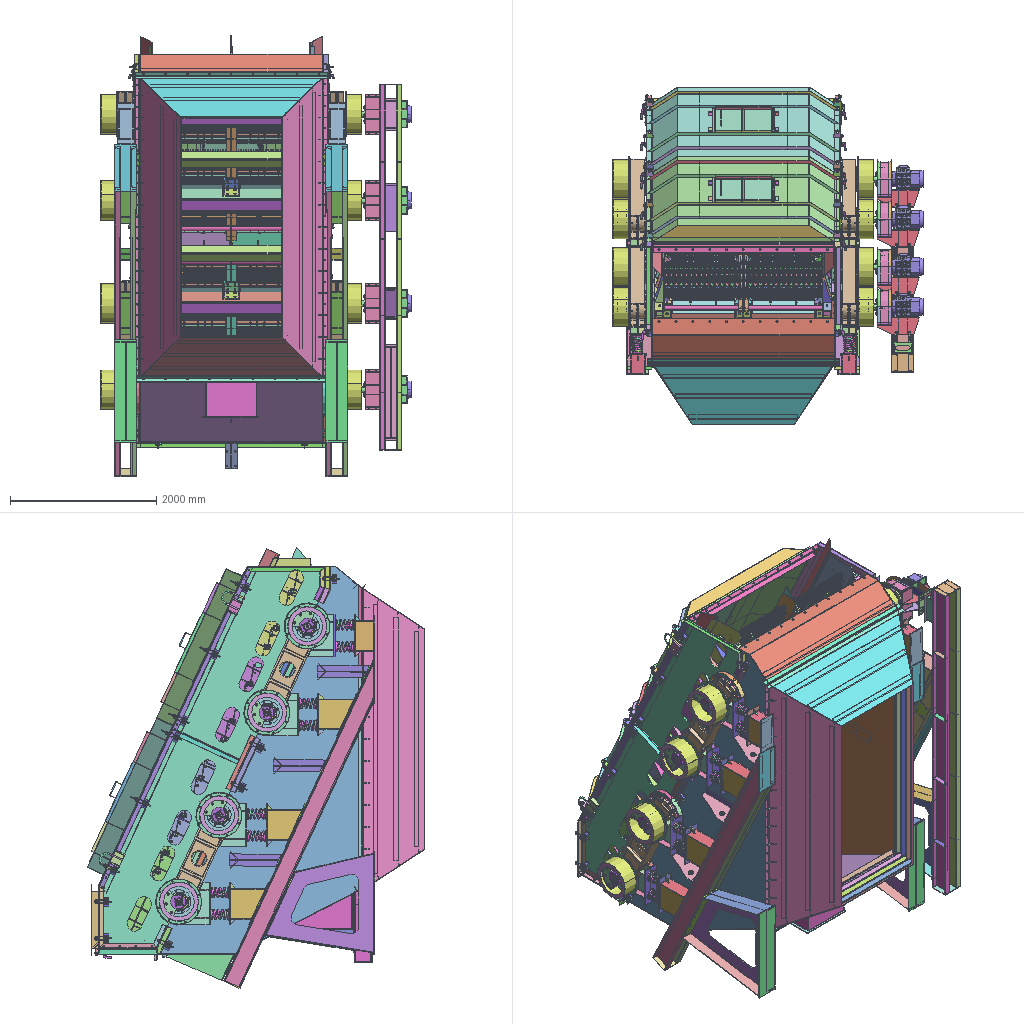Assembly | STEP file | 152 different items | 6490 placed | box 4240 x 4616 x 6023 mm
Parts list (item | name | quantity | parent item | size | volume):
1 | Side plate assembly 2_Default<As machined> | x2 | in Lower hopper | 630.687 x 850.025 x 4105 mm | 42475037 mm3
2 | Rear baffle assembly 2_Default<As machined> | x1 | in Lower hopper | 2450 x 950 x 83 mm | 21025838 mm3
3 | Front baffle assembly 2_Default<As machined> | x1 | in Lower hopper | 2450 x 950 x 83 mm | 21006283 mm3
4 | Angle steel L63X63X8-2626_Default<As machined> | x2 | in Lower hopper | 2626 x 63 x 63 mm | 2498543 mm3
5 | Screen frame side plate assembly_Default<As machined> | x1 | in Upper hopper assembly | 5295 x 2809 x 83 mm | 63364081 mm3
6 | Mirror screen frame side plate assembly_Default<As machined><As machined> | x1 | in Upper hopper assembly | 5295 x 2809 x 83 mm | 63364081 mm3
7 | Positioning angle steel_Default<As machined> | x1 | in Upper hopper assembly | 83 x 58 x 2484 mm | 2642976 mm3
8 | Edge support_Default<As machined> | x3 | in Upper hopper assembly | 168.631 x 720.909 x 332 mm | 2997743 mm3
9 | Mirror edge support_Default<As machined><As machined> | x3 | in Upper hopper assembly | 168.631 x 720.909 x 332 mm | 2997743 mm3
10 | Front baffle_Default<As machined> | x1 | in Upper hopper assembly | 304.499 x 630.195 x 2626 mm | 17251422 mm3
11 | Upper hopper rear baffle_Default<As machined> | x1 | in Upper hopper assembly | 1001 x 2838 x 2626 mm | 60427980 mm3
12 | Screen frame rear support_Default<As machined> | x1 | in Upper hopper assembly | 426.209 x 826.5 x 160 mm | 3581140 mm3
13 | Angle steel L160X60X10-2484_Default<As machined> | x3 | in Upper hopper assembly | 2484 x 226.274 x 118.827 mm | 7825020 mm3
14 | Maintenance pipe_Default<As machined> | x1 | in Hopper assembly | 740 x 860 x 475 mm | 8939485 mm3
15 | Door_Default<As machined> | x1 | in Hopper assembly | 740 x 860 x 74 mm | 3877047 mm3
16 | GN 128.2-120-A41201611203204 | x2 | in Hopper assembly | 20 x 120 x 16 mm | 25167 mm3
17 | Rubber pad_Default<As machined> | x32 | in Spring seat assembly, Spring seat assembly 2 | 160 x 160 x 8 mm | 104144 mm3
18 | Spring lower seat 1_Default<As machined> | x6 | in Spring seat assembly | 580.577 x 601.953 x 230 mm | 9576180 mm3
19 | Helical spring_22X120X280 stiffness 222 | x16 | in Spring seat assembly, Spring seat assembly 2 | 142 x 142 x 244.587 mm | 741236 mm3
20 | Spring upper seat (I)_Default<As machined> | x8 | in Spring seat assembly, Spring seat assembly 2 | 580.577 x 439.316 x 230 mm | 6180967 mm3
21 | Spring lower seat 2_Default<As machined> | x2 | in Spring seat assembly 2 | 575.505 x 341 x 230 mm | 7946213 mm3
22 | _1-QC-408710.step | x27 | in Horizontal tension series latch quick clamp [QC-408710].step | 62 x 37 x 74.9 mm | 22748 mm3
23 | _2-QC-408710.step | x27 | in Horizontal tension series latch quick clamp [QC-408710].step | 60 x 71.267 x 120.088 mm | 53013 mm3
24 | _3-QC-408710.step | x27 | in Horizontal tension series latch quick clamp [QC-408710].step | 57.17 x 14.63 x 155.83 mm | 19518 mm3
25 | _4-QC-408710.step | x27 | in Horizontal tension series latch quick clamp [QC-408710].step | 28 x 37.92 x 40 mm | 9998 mm3
26 | Part 5 | x30 | in Horizontal tension series latch quick clamp [QC-408710], Rear baffle assembly | 126 x 61 x 55 mm | 39850 mm3
27 | Lower channel steel_Default<As machined> | x2 | in Screen frame component assembly | 4891 x 283.464 x 300 mm | 35069262 mm3
28 | Leg_Default<As machined> | x2 | in Screen frame component assembly | 1400 x 1507 x 300 mm | 26750230 mm3
29 | Side plate_Default<As machined> | x1 | in Side plate assembly | 6040 x 1090 x 73 mm | 39402271 mm3
30 | Part 4_Default<As machined> | x1 | in Side plate assembly | 6040 x 1090 x 81 mm | 13497618 mm3
31 | Part 5_Default<As machined> | x14 | in Side plate assembly, Feed inlet assembly, Rear baffle assembly | 82 x 30 x 10 mm | 22938 mm3
32 | Hanger_Default<As machined> | x2 | in Side plate assembly | 190 x 295 x 20 mm | 209555 mm3
33 | Mirror side plate_Default<As machined><As machined> | x1 | in Mirror side plate assembly | 6040 x 1090 x 73 mm | 39402271 mm3
34 | Mirror part 4_Default<As machined> | x1 | in Mirror side plate assembly | 6040 x 1090 x 81 mm | 13497621 mm3
35 | Mirror part 5_Default<As machined><As machined> | x4 | in Mirror side plate assembly | 82 x 30 x 10 mm | 22938 mm3
36 | Mirror hanger_Default<As machined><As machined> | x2 | in Mirror side plate assembly | 190 x 295 x 20 mm | 209555 mm3
37 | Connecting beam 1_Default<As machined> | x1 | in Screen box assembly | 214 x 150.815 x 2484 mm | 9468856 mm3
38 | Connecting beam 2_Default<As machined> | x1 | in Screen box assembly | 2484 x 75 x 180 mm | 5664884 mm3
39 | Connecting beam 3_Default<As machined> | x1 | in Screen box assembly | 255.713 x 102 x 2484 mm | 8118407 mm3
40 | Feed inlet flange_Default<As machined> | x1 | in Feed inlet assembly | 1960 x 960 x 10 mm | 4768318 mm3
41 | Bottom plate 6_Default<As machined> | x1 | in Feed inlet assembly | 934 x 2650 x 6 mm | 6458664 mm3
42 | Liner plate_Default<As machined> | x1 | in Feed inlet assembly | 260 x 1764 x 16 mm | 7243869 mm3
43 | Rear bottom plate_Default<As machined> | x1 | in Feed inlet assembly | 260 x 1784 x 10 mm | 4607815 mm3
44 | Plate 1784X80X8_Default<As machined> | x2 | in Feed inlet assembly | 1784 x 100 x 8 mm | 1427200 mm3
45 | Part 8 | x2 | in Feed inlet assembly | 208 x 768 x 8 mm | 1182208 mm3
46 | GB/T 70.3-2000 hex socket countersunk screw M16×50 (8.8 grade) | x12 | in Feed inlet assembly | 50 x 33.6 x 33.6 mm | 12258 mm3
47 | GB/T 95-2002 flat washer, grade C 16×3 (steel) | x52 | in Feed inlet assembly, Screen box assembly, Exciter assembly | 30 x 3 x 30 mm | 1399 mm3
48 | GB/T 93-1987 standard spring washer (assembly) 16×4.1 (65Mn) | x52 | in Feed inlet assembly, Screen box assembly, Exciter assembly | 24.356 x 24.313 x 4.1 mm | 1031 mm3
49 | GB/T 41-20001 hex nut, grade C, M16 (4 grade) | x20 | in Feed inlet assembly, Screen box assembly | 26.17 x 22.664 x 15.9 mm | 3864 mm3
50 | Rear baffle_Default<As machined> | x1 | in Rear baffle assembly | 150 x 800 x 2650 mm | 24404542 mm3
51 | Seal cover 2_Default<As machined> | x1 | in Screen box assembly | 2723 x 292.121 x 2296 mm | 30393848 mm3
52 | Seal cover 1_Default<As machined> | x1 | in Screen box assembly | 2723 x 286.121 x 2250 mm | 29731618 mm3
53 | Manhole door_Default<As machined> | x2 | in Screen box assembly | 840 x 840 x 140 mm | 3861650 mm3
54 | _PDHFA1-75.step | x4 | in Welded hinge, square, A series [PDHFA-75].step | 29.25 x 8.5 x 75 mm | 5922 mm3
55 | _PDHFA2-75.step | x4 | in Welded hinge, square, A series [PDHFA-75].step | 29.25 x 8.5 x 75 mm | 5070 mm3
56 | GB/T 5781-2000 hex head bolt, fully threaded, grade C M16×45 (3.6 grade) | x8 | in Screen box assembly | 55 x 27.713 x 24 mm | 13928 mm3
57 | Screen plate bracket (middle 1)_Default<As machined> | x1 | in Screen plate bracket in | 3120 x 451.736 x 230 mm | 29285833 mm3
58 | Screen plate bracket (edge)_Default<As machined> | x4 | in Screen plate bracket in, Screen plate bracket out | 2750 x 152 x 230 mm | 16995025 mm3
59 | Square tube 120X120X8-1079_Default<As machined> | x8 | in Screen plate bracket in, Screen plate bracket out | 1079 x 120 x 120 mm | 3686687 mm3
60 | Gusset plate 1_Default<As machined> | x32 | in Screen plate bracket in, Screen plate bracket out | 60 x 100 x 12 mm | 54600 mm3
61 | - | x4 | in Screen plate bracket in, Screen plate bracket out | 2404 x 70 x 70 mm | 3745985 mm3
62 | Beam guard plate_Default<As machined> | x8 | in Screen plate bracket in, Screen plate bracket out | 305.019 x 262.777 x 850 mm | 2327560 mm3
63 | GB/T 5783-2000 hex head bolt, fully threaded M10×45 (5.6 grade) | x64 | in Screen plate bracket in, Screen plate bracket out, Exciter assembly | 31.4 x 18.475 x 16 mm | 3346 mm3
64 | GB/T 93-1987 standard spring washer (assembly) 10×2.6 (65Mn) | x64 | in Screen plate bracket in, Screen plate bracket out, Exciter assembly | 15.372 x 15.344 x 2.6 mm | 261.313 mm3
65 | GB/T 95-2002 flat washer, grade C 10×2 (steel) | x64 | in Screen plate bracket in, Screen plate bracket out, Exciter assembly | 20 x 2 x 20 mm | 438.252 mm3
66 | Screen plate bracket (middle 2)_Default<As machined> | x1 | in Screen plate bracket out | 2936 x 451.736 x 230 mm | 28253471 mm3
67 | Motor bracket lower channel steel_Default<As machined> | x1 | in Motor bracket assembly | 5000 x 250 x 300 mm | 37542692 mm3
68 | Motor bracket leg_Default<As machined> | x1 | in Motor bracket assembly | 1300 x 1259 x 300 mm | 22043993 mm3
69 | Motor base_Default<As machined> | x4 | in Assembly 3, Motor bracket assembly | 572.5 x 250 x 550 mm | 5315088 mm3
70 | Motor lower seat 1_Default<As machined> | x3 | in Assembly 3 | 436 x 591.846 x 300 mm | 6753859 mm3
71 | GB/T901-1988 double-end stud, grade B, M24×300 | x12 | in Assembly 3 | 300 x 24 x 24 mm | 120071 mm3
72 | GB/T41-20001 hex nut, grade C, M24 | x64 | in Assembly 3, Motor bracket assembly | 39.55 x 34.251 x 22.3 mm | 12527 mm3
73 | Coupling guard_Default<As machined> | x4 | in Assembly 3, Motor bracket assembly | 550 x 522 x 200 mm | 1395194 mm3
74 | Motor base support channel steel_Default<As machined> | x1 | in Motor bracket assembly | 3569 x 291.917 x 300 mm | 27407962 mm3
75 | Motor lower seat 2_Default<As machined> | x1 | in Motor bracket assembly | 436 x 154.533 x 300 mm | 3621040 mm3
76 | GB/T901-1988 double-end stud, grade B, M24×200 | x4 | in Motor bracket assembly | 200 x 24 x 24 mm | 86144 mm3
77 | Rectangular tube | x4 | in Rectangular tube beam | 239 x 320 x 2600 mm | 50963884 mm3
78 | Flange | x8 | in Rectangular tube beam | 34 x 476 x 476 mm | 2924692 mm3
79 | Plate 510x230x16 | x4 | in Rectangular tube beam | 510 x 2414 x 16 mm | 5441904 mm3
80 | GB/T 5783-2000 hex head bolt, fully threaded, M20×40 (5.6 grade) | x8 | in Rectangular tube beam | 52.5 x 34.641 x 30 mm | 22112 mm3
81 | Rib 9 | x16 | in Rectangular tube beam | 60 x 60 x 12 mm | 27600 mm3
82 | Rib 7 | x16 | in Rectangular tube beam | 150 x 60 x 12 mm | 77400 mm3
83 | Reinforcing plate 4 | x24 | in Rectangular tube beam | 230 x 230 x 12 mm | 600871 mm3
84 | Rib 6 | x48 | in Rectangular tube beam | 123 x 230 x 12 mm | 222480 mm3
85 | Drive shaft | x4 | in Exciter assembly | 3402 x 140 x 140 mm | 19524168 mm3
86 | Oil retaining ring | x8 | in Exciter assembly | 41.5 x 216 x 216 mm | 640315 mm3
87 | GB/T1096-1979 plain key, type A, 24×90 | x8 | in Exciter assembly | 90 x 24 x 14 mm | 28453 mm3
88 | End disc | x8 | in Exciter assembly | 620 x 620 x 4 mm | 989174 mm3
89 | Labyrinth cover | x8 | in Exciter assembly | 65 x 227.5 x 227.5 mm | 634652 mm3
90 | Offset block | x8 | in Offset block assembly | 424.352 x 335 x 125 mm | 6174570 mm3
91 | Part 7 | x24 | in Offset block assembly | 389.711 x 169 x 20 mm | 776785 mm3
92 | GB/T 5780-2000 hex head bolt, grade C, M20×120 (3.6 grade) | x24 | in Offset block assembly | 132.5 x 34.641 x 30 mm | 47244 mm3
93 | GB/T 93-1987 standard spring washer (assembly) 20×5 (65Mn) | x32 | in Offset block assembly, Exciter assembly | 30.149 x 30.097 x 5 mm | 1905 mm3
94 | Through-hole cover | x8 | in Exciter assembly | 49 x 330 x 330 mm | 1508672 mm3
95 | Shaft end baffle | x8 | in Exciter assembly | 20 x 95 x 95 mm | 108579 mm3
96 | Taper sleeve | x8 | in Exciter assembly | 120 x 95 x 94.958 mm | 185425 mm3
97 | Bearing housing | x4 | in Exciter assembly | 1820 x 234 x 460 mm | 47518256 mm3
98 | GB/T288-94 spherical roller bearing 22324C_1 | x8 | in Exciter assembly | 86 x 260 x 260 mm | 2801542 mm3
99 | JB1091-1991 skeleton-type vacuum rubber seal ring 140 | x8 | in Exciter assembly | 170 x 16 x 170 mm | 62160 mm3
100 | GB/T 5786-2000 hex head bolt, fine thread, fully threaded, grade A and B, M24×60 (5.6 grade) | x8 | in Exciter assembly | 75 x 41.569 x 36 mm | 43647 mm3
101 | GB/T 93-1987 standard spring washer (assembly) 24×6 (65Mn) | x72 | in Exciter assembly | 36.439 x 36.377 x 6 mm | 3321 mm3
102 | Guard cover | x8 | in Exciter assembly | 620 x 620 x 220 mm | 2105294 mm3
103 | GB/T 5780-2000 hex head bolt, grade C, M24×100 (3.6 grade) | x64 | in Exciter assembly | 115 x 41.569 x 36 mm | 61742 mm3
104 | GB/T 95-2002 flat washer, grade C 24×4 (steel) | x64 | in Exciter assembly | 44 x 4 x 44 mm | 3958 mm3
105 | GB/T 41-20001 hex nut, grade C, M24 (4 grade) | x64 | in Exciter assembly | 39.55 x 34.251 x 22.3 mm | 12527 mm3
106 | GB/T 5781-2000 hex head bolt, fully threaded, grade C, M12×45 (3.6 grade) | x64 | in Exciter assembly | 52.5 x 20.785 x 18 mm | 7141 mm3
107 | GB/T 93-1987 standard spring washer (assembly) 12×3.1 (65Mn) | x64 | in Exciter assembly | 18.367 x 18.334 x 3.1 mm | 444.091 mm3
108 | GB/T 41-20001 hex nut, grade C, M10 (4 grade) | x32 | in Exciter assembly | 17.59 x 15.233 x 9.5 mm | 1159 mm3
109 | Coupling | x4 | in Exciter assembly | 157 x 250 x 250 mm | 2335528 mm3
110 | GB/T 5780-2000 hex head bolt, grade C, M20×80 (3.6 grade) | x8 | in Exciter assembly | 92.5 x 34.641 x 30 mm | 34678 mm3
111 | GB/T 95-2002 flat washer, grade C 20×3 (steel) | x8 | in Exciter assembly | 37 x 3 x 37 mm | 2085 mm3
112 | Coupling 2 | x4 | in Exciter assembly | 104 x 250 x 250 mm | 1439037 mm3
113 | Coupling rubber strip | x16 | in Exciter assembly | 129 x 167.5 x 80 mm | 367054 mm3
114 | Pressing pad | x32 | in Exciter assembly | 60 x 60 x 10 mm | 25730 mm3
115 | GB/T 5780-2000 hex head bolt, grade C, M16×65 (3.6 grade) | x32 | in Exciter assembly | 75 x 27.713 x 24 mm | 17949 mm3
116 | IM B3 H63-132 variable-frequency motor [YVF2-132S2-4-B3]_YVF2-132S2-4-B3 | x4 | in 1233 | 270 x 315 x 510 mm | 20221478 mm3
117 | Grid blind plate_Default<As machined> | x2 | in Bar screen plate 1 | 874.382 x 165 x 1059 mm | 15878057 mm3
118 | Positioning slot assembly 1_Default<As machined> | x30 | in Bar screen assembly 1 | 100 x 92 x 1069 mm | 2012408 mm3
119 | - | x930 | in Bar screen assembly 1 | 10 x 10 x 340 mm | 26704 mm3
120 | - | x930 | in Bar screen assembly 1 | 10 x 10 x 310 mm | 24347 mm3
121 | - | x2610 | in Bar screen assembly 1 | 8 x 8 x 310 mm | 15582 mm3
122 | Pressure plate 1069X36X6_Default<As machined> | x30 | in Bar screen assembly 1 | 1069 x 6 x 36 mm | 230904 mm3
123 | GB/T5783-2000 hex head bolt, fully threaded M10×45 | x180 | in Bar screen assembly 1 | 51.4 x 18.475 x 16 mm | 4917 mm3
124 | Rear baffle 1079X402X8_Default<As machined> | x2 | in Bar screen plate 1 | 1079 x 402 x 8 mm | 3470064 mm3
125 | - | x84 | in Bar screen plate 1, Bar screen plate 2, Bar screen plate 3, Bar screen plate 4 | 36 x 36 x 280 mm | 87085 mm3
126 | - | x28 | in Bar screen plate 1, Bar screen plate 2, Bar screen plate 3, Bar screen plate 4 | 16 x 16 x 1069 mm | 214935 mm3
127 | Connecting plate assembly 1_Default<As machined> | x4 | in Bar screen plate 1 | 725.342 x 86.845 x 24 mm | 319823 mm3
128 | Edge plate 1_Default<As machined> | x1 | in Bar screen plate 1 | 1555 x 210 x 35 mm | 3116927 mm3
129 | Edge plate 2_Default<As machined> | x1 | in Bar screen plate 1 | 130 x 532.359 x 1587 mm | 10246266 mm3
130 | Rubber plate 1_Default<As machined> | x2 | in Bar screen plate 1 | 1355 x 250 x 8 mm | 2297597 mm3
131 | Mirror edge plate 1_Default<As machined><As machined> | x1 | in Bar screen plate 1 | 1555 x 210 x 35 mm | 3116927 mm3
132 | Mirror edge plate 2_Default<As machined><As machined> | x1 | in Bar screen plate 1 | 130 x 532.359 x 1587 mm | 10246266 mm3
133 | Connecting plate assembly 2_Default<As machined> | x4 | in Bar screen plate 2 | 1223 x 86.845 x 24 mm | 635186 mm3
134 | Edge plate 3_Default<As machined> | x1 | in Bar screen plate 2 | 1554 x 210 x 35 mm | 2937527 mm3
135 | Edge plate 4_Default<As machined> | x1 | in Bar screen plate 2 | 207.636 x 532.359 x 1552 mm | 10466658 mm3
136 | Rubber plate 2_Default<As machined> | x6 | in Bar screen plate 2, Bar screen plate 3, Bar screen plate 4 | 1374 x 250 x 8 mm | 2740611 mm3
137 | Pressure plate 2_Default<As machined> | x6 | in Bar screen plate 2, Bar screen plate 3, Bar screen plate 4 | 1374 x 40 x 4 mm | 216145 mm3
138 | Bent plate 1_Default<As machined> | x1 | in Bar screen plate 2 | 330 x 204.897 x 1059 mm | 4219235 mm3
139 | Liner plate 1_Default<As machined> | x2 | in Bar screen plate 2 | 330 x 1049 x 8 mm | 2695509 mm3
140 | Mirror edge plate 3_Default<As machined><As machined> | x1 | in Bar screen plate 2 | 1554 x 210 x 35 mm | 2937527 mm3
141 | Mirror bent plate 1_Default<As machined><As machined> | x1 | in Bar screen plate 2 | 330 x 204.897 x 1059 mm | 4219235 mm3
142 | Mirror edge plate 4_Default<As machined><As machined> | x1 | in Bar screen plate 2 | 207.636 x 532.359 x 1552 mm | 10466658 mm3
143 | Edge plate 5_Default<As machined> | x1 | in Bar screen plate 3 | 1374 x 260 x 35 mm | 3099117 mm3
144 | Edge plate 6_Default<As machined> | x1 | in Bar screen plate 3 | 130 x 532.359 x 1374 mm | 9676363 mm3
145 | Connecting plate assembly 3_Default<As machined> | x4 | in Bar screen plate 3 | 1250 x 86.845 x 24 mm | 582349 mm3
146 | Mirror edge plate 5_Default<As machined><As machined> | x1 | in Bar screen plate 3 | 1374 x 260 x 35 mm | 3099117 mm3
147 | Mirror edge plate 6_Default<As machined><As machined> | x1 | in Bar screen plate 3 | 130 x 532.359 x 1374 mm | 9676363 mm3
148 | Edge plate 7_Default<As machined> | x1 | in Bar screen plate 4 | 1511 x 260 x 35 mm | 3690417 mm3
149 | Edge plate 8_Default<As machined> | x1 | in Bar screen plate 4 | 130 x 532.359 x 1511 mm | 9898489 mm3
150 | Bar screen plate 4_Default<As machined> | x4 | in Bar screen plate 4 | 1234 x 86.845 x 24 mm | 638578 mm3
151 | Mirror edge plate 7_Default<As machined><As machined> | x1 | in Bar screen plate 4 | 1511 x 260 x 35 mm | 3690417 mm3
152 | Mirror edge plate 8_Default<As machined><As machined> | x1 | in Bar screen plate 4 | 130 x 532.359 x 1511 mm | 9898489 mm3
Placements (level | parent | child | x y z in mm | rotation matrix by rows), first 266 of 6622 lines:
1 | 1233 | Screen frame component assembly | -0.0 -0.0 -0.0 | 1 0 0 0 1 0 0 0 1
2 | Screen frame component assembly | Hopper assembly | -0.0 -0.0 -0.0 | 1 0 0 0 1 0 0 0 1
3 | Hopper assembly | Lower hopper | -0.0 -0.0 -0.0 | 1 0 0 0 1 0 0 0 1
4 | Lower hopper | Side plate assembly 2_Default<As machined> | 1313.0 -8.0 0.0 | 1 0 0 0 1 0 0 0 1
4 | Lower hopper | Rear baffle assembly 2_Default<As machined> | 0.0 -850.025 1509.541 | -1 0 0 0 0.8385 0.545 0 0.545 -0.8385
4 | Lower hopper | Front baffle assembly 2_Default<As machined> | 0.0 -850.025 -1509.541 | 1 0 0 0 0.8385 0.545 0 -0.545 0.8385
4 | Lower hopper | Side plate assembly 2_Default<As machined> | -1313.0 -8.0 0.0 | -1 0 0 0 1 0 0 0 -1
4 | Lower hopper | Angle steel L63X63X8-2626_Default<As machined> | 0.0 -0.0 2062.041 | 1 0 0 0 -0.545 -0.8385 0 0.8385 -0.545
4 | Lower hopper | Angle steel L63X63X8-2626_Default<As machined> | -0.0 -0.0 -2062.041 | -1 0 0 0 -0.545 -0.8385 0 -0.8385 0.545
3 | Hopper assembly | Upper hopper assembly | -4045.416 1401.429 -250.506 | 0 0 1 0 1 0 -1 0 0
4 | Upper hopper assembly | Screen frame side plate assembly_Default<As machined> | 1791.123 -1401.429 5295.416 | 1 0 0 0 1 0 0 0 1
4 | Upper hopper assembly | Mirror screen frame side plate assembly_Default<As machined><As machined> | 1791.123 -1401.429 2795.416 | 1 0 0 0 1 0 0 0 1
4 | Upper hopper assembly | Positioning angle steel_Default<As machined> | -0.0 -0.0 -0.0 | 1 0 0 0 1 0 0 0 1
4 | Upper hopper assembly | Edge support_Default<As machined> | -1176.285 -781.042 2791.416 | -1 -0.006557 0 -0.006557 1 0 0 0 -1
4 | Upper hopper assembly | Edge support_Default<As machined> | 110.808 -180.861 2791.416 | -1 -0.006557 0 -0.006557 1 0 0 0 -1
4 | Upper hopper assembly | Edge support_Default<As machined> | 1397.9 419.32 2791.416 | -1 -0.006557 0 -0.006557 1 0 0 0 -1
4 | Upper hopper assembly | Mirror edge support_Default<As machined><As machined> | 1397.9 419.32 5299.416 | -1 -0.006557 0 -0.006557 1 0 0 0 -1
4 | Upper hopper assembly | Mirror edge support_Default<As machined><As machined> | 110.808 -180.861 5299.416 | -1 -0.006557 0 -0.006557 1 0 0 0 -1
4 | Upper hopper assembly | Mirror edge support_Default<As machined><As machined> | -1176.285 -781.042 5299.416 | -1 -0.006557 0 -0.006557 1 0 0 0 -1
4 | Upper hopper assembly | Front baffle_Default<As machined> | -2611.106 -810.792 4045.416 | -1 0 0 0 1 0 0 0 -1
4 | Upper hopper assembly | Upper hopper rear baffle_Default<As machined> | 2684.309 1407.529 4045.416 | 1 0 0 0 1 0 0 0 1
4 | Upper hopper assembly | Screen frame rear support_Default<As machined> | 3042.855 530.716 4045.416 | -0.9011 -0.4335 0 -0.4335 0.9011 0 0 0 -1
4 | Upper hopper assembly | Angle steel L160X60X10-2484_Default<As machined> | -1175.446 -909.02 4045.416 | 0 -1 -0.006557 0 -0.006557 1 -1 0 0
4 | Upper hopper assembly | Angle steel L160X60X10-2484_Default<As machined> | 111.647 -308.839 4045.416 | 0 -1 -0.006557 0 -0.006557 1 -1 0 0
4 | Upper hopper assembly | Angle steel L160X60X10-2484_Default<As machined> | 1398.74 291.343 4045.416 | 0 -1 -0.006557 0 -0.006557 1 -1 0 0
3 | Hopper assembly | Maintenance pipe_Default<As machined> | -0.0 541.628 -2591.349 | 1 0 0 0 1 0 0 0 1
3 | Hopper assembly | Door_Default<As machined> | -0.0 541.628 -2591.349 | -1 0 0 0 1 0 0 0 -1
3 | Hopper assembly | GN 128.2-120-A41201611203204 | 358.0 823.128 -2589.349 | -0.6 0 0.8 0 -1 0 0.8 0 0.6
3 | Hopper assembly | GN 128.2-120-A41201611203204 | 358.0 260.128 -2589.349 | -0.6 0 0.8 0 -1 0 0.8 0 0.6
2 | Screen frame component assembly | Spring seat assembly | -1442.0 617.014 337.6 | 0 0 1 0 1 0 -1 0 0
3 | Spring seat assembly | Rubber pad_Default<As machined> | -150.0 -0.0 0.0 | -0.03619 0.9993 0 0 0 1 0.9993 0.03619 0
3 | Spring seat assembly | Spring lower seat 1_Default<As machined> | 0.0 -0.0 -0.0 | -1 0 0 0 1 0 0 0 -1
3 | Spring seat assembly | Helical spring_22X120X280 stiffness 222 | -150.0 2.473 -0.0 | -0.008683 1 0 0 0 1 1 0.008683 0
3 | Spring seat assembly | Helical spring_22X120X280 stiffness 222 | 150 2.473 -0.0061 | -0.008683 -1 0 0 0 1 -1 0.008683 0
3 | Spring seat assembly | Rubber pad_Default<As machined> | 150.0 8.0 0.0 | 0.03619 -0.9993 0 0 0 -1 0.9993 0.03619 -0
3 | Spring seat assembly | Rubber pad_Default<As machined> | -150.0 252.587 0.0 | -0.03619 0.9993 0 0 0 1 0.9993 0.03619 0
3 | Spring seat assembly | Rubber pad_Default<As machined> | 150.0 260.587 0.0 | 0.03619 -0.9993 0 0 0 -1 0.9993 0.03619 -0
3 | Spring seat assembly | Spring upper seat (I)_Default<As machined> | 0.0 260.587 -0.0 | -1 0 0 0 1 0 0 0 -1
2 | Screen frame component assembly | Spring seat assembly | -1442.0 1320.672 -1171.4 | 0 0 1 0 1 0 -1 0 0
3 | Spring seat assembly | Rubber pad_Default<As machined> | -150.0 -0.0 0.0 | -0.03619 0.9993 0 0 0 1 0.9993 0.03619 0
3 | Spring seat assembly | Spring lower seat 1_Default<As machined> | 0.0 -0.0 -0.0 | -1 0 0 0 1 0 0 0 -1
3 | Spring seat assembly | Helical spring_22X120X280 stiffness 222 | -150.0 2.473 -0.0 | -0.008683 1 0 0 0 1 1 0.008683 0
3 | Spring seat assembly | Helical spring_22X120X280 stiffness 222 | 150 2.473 -0.0061 | -0.008683 -1 0 0 0 1 -1 0.008683 0
3 | Spring seat assembly | Rubber pad_Default<As machined> | 150.0 8.0 0.0 | 0.03619 -0.9993 0 0 0 -1 0.9993 0.03619 -0
3 | Spring seat assembly | Rubber pad_Default<As machined> | -150.0 252.587 0.0 | -0.03619 0.9993 0 0 0 1 0.9993 0.03619 0
3 | Spring seat assembly | Rubber pad_Default<As machined> | 150.0 260.587 0.0 | 0.03619 -0.9993 0 0 0 -1 0.9993 0.03619 -0
3 | Spring seat assembly | Spring upper seat (I)_Default<As machined> | 0.0 260.587 -0.0 | -1 0 0 0 1 0 0 0 -1
2 | Screen frame component assembly | Spring seat assembly | -1442.0 1821.487 -2245.4 | 0 0 1 0 1 0 -1 0 0
3 | Spring seat assembly | Rubber pad_Default<As machined> | -150.0 -0.0 0.0 | -0.03619 0.9993 0 0 0 1 0.9993 0.03619 0
3 | Spring seat assembly | Spring lower seat 1_Default<As machined> | 0.0 -0.0 -0.0 | -1 0 0 0 1 0 0 0 -1
3 | Spring seat assembly | Helical spring_22X120X280 stiffness 222 | -150.0 2.473 -0.0 | -0.008683 1 0 0 0 1 1 0.008683 0
3 | Spring seat assembly | Helical spring_22X120X280 stiffness 222 | 150 2.473 -0.0061 | -0.008683 -1 0 0 0 1 -1 0.008683 0
3 | Spring seat assembly | Rubber pad_Default<As machined> | 150.0 8.0 0.0 | 0.03619 -0.9993 0 0 0 -1 0.9993 0.03619 -0
3 | Spring seat assembly | Rubber pad_Default<As machined> | -150.0 252.587 0.0 | -0.03619 0.9993 0 0 0 1 0.9993 0.03619 0
3 | Spring seat assembly | Rubber pad_Default<As machined> | 150.0 260.587 0.0 | 0.03619 -0.9993 0 0 0 -1 0.9993 0.03619 -0
3 | Spring seat assembly | Spring upper seat (I)_Default<As machined> | 0.0 260.587 -0.0 | -1 0 0 0 1 0 0 0 -1
2 | Screen frame component assembly | Spring seat assembly | 1442.0 1821.487 -2245.4 | 0 0 1 0 1 0 -1 0 -0
3 | Spring seat assembly | Rubber pad_Default<As machined> | -150.0 -0.0 0.0 | -0.03619 0.9993 0 0 0 1 0.9993 0.03619 0
3 | Spring seat assembly | Spring lower seat 1_Default<As machined> | 0.0 -0.0 -0.0 | -1 0 0 0 1 0 0 0 -1
3 | Spring seat assembly | Helical spring_22X120X280 stiffness 222 | -150.0 2.473 -0.0 | -0.008683 1 0 0 0 1 1 0.008683 0
3 | Spring seat assembly | Helical spring_22X120X280 stiffness 222 | 150 2.473 -0.0061 | -0.008683 -1 0 0 0 1 -1 0.008683 0
3 | Spring seat assembly | Rubber pad_Default<As machined> | 150.0 8.0 0.0 | 0.03619 -0.9993 0 0 0 -1 0.9993 0.03619 -0
3 | Spring seat assembly | Rubber pad_Default<As machined> | -150.0 252.587 0.0 | -0.03619 0.9993 0 0 0 1 0.9993 0.03619 0
3 | Spring seat assembly | Rubber pad_Default<As machined> | 150.0 260.587 0.0 | 0.03619 -0.9993 0 0 0 -1 0.9993 0.03619 -0
3 | Spring seat assembly | Spring upper seat (I)_Default<As machined> | 0.0 260.587 -0.0 | -1 0 0 0 1 0 0 0 -1
2 | Screen frame component assembly | Spring seat assembly | 1442.0 1320.672 -1171.4 | 0 0 1 0 1 0 -1 0 -0
3 | Spring seat assembly | Rubber pad_Default<As machined> | -150.0 -0.0 0.0 | -0.03619 0.9993 0 0 0 1 0.9993 0.03619 0
3 | Spring seat assembly | Spring lower seat 1_Default<As machined> | 0.0 -0.0 -0.0 | -1 0 0 0 1 0 0 0 -1
3 | Spring seat assembly | Helical spring_22X120X280 stiffness 222 | -150.0 2.473 -0.0 | -0.008683 1 0 0 0 1 1 0.008683 0
3 | Spring seat assembly | Helical spring_22X120X280 stiffness 222 | 150 2.473 -0.0061 | -0.008683 -1 0 0 0 1 -1 0.008683 0
3 | Spring seat assembly | Rubber pad_Default<As machined> | 150.0 8.0 0.0 | 0.03619 -0.9993 0 0 0 -1 0.9993 0.03619 -0
3 | Spring seat assembly | Rubber pad_Default<As machined> | -150.0 252.587 0.0 | -0.03619 0.9993 0 0 0 1 0.9993 0.03619 0
3 | Spring seat assembly | Rubber pad_Default<As machined> | 150.0 260.587 0.0 | 0.03619 -0.9993 0 0 0 -1 0.9993 0.03619 -0
3 | Spring seat assembly | Spring upper seat (I)_Default<As machined> | 0.0 260.587 -0.0 | -1 0 0 0 1 0 0 0 -1
2 | Screen frame component assembly | Spring seat assembly | 1442.0 617.014 337.6 | 0 0 1 0 1 0 -1 0 -0
3 | Spring seat assembly | Rubber pad_Default<As machined> | -150.0 -0.0 0.0 | -0.03619 0.9993 0 0 0 1 0.9993 0.03619 0
3 | Spring seat assembly | Spring lower seat 1_Default<As machined> | 0.0 -0.0 -0.0 | -1 0 0 0 1 0 0 0 -1
3 | Spring seat assembly | Helical spring_22X120X280 stiffness 222 | -150.0 2.473 -0.0 | -0.008683 1 0 0 0 1 1 0.008683 0
3 | Spring seat assembly | Helical spring_22X120X280 stiffness 222 | 150 2.473 -0.0061 | -0.008683 -1 0 0 0 1 -1 0.008683 0
3 | Spring seat assembly | Rubber pad_Default<As machined> | 150.0 8.0 0.0 | 0.03619 -0.9993 0 0 0 -1 0.9993 0.03619 -0
3 | Spring seat assembly | Rubber pad_Default<As machined> | -150.0 252.587 0.0 | -0.03619 0.9993 0 0 0 1 0.9993 0.03619 0
3 | Spring seat assembly | Rubber pad_Default<As machined> | 150.0 260.587 0.0 | 0.03619 -0.9993 0 0 0 -1 0.9993 0.03619 -0
3 | Spring seat assembly | Spring upper seat (I)_Default<As machined> | 0.0 260.587 -0.0 | -1 0 0 0 1 0 0 0 -1
2 | Screen frame component assembly | Spring seat assembly 2 | -1442.0 116.975 1411.6 | 0 0 1 0 1 0 -1 0 0
3 | Spring seat assembly 2 | Rubber pad_Default<As machined> | -150.0 0.0 0.0 | -0.03619 0.9993 0 0 0 1 0.9993 0.03619 0
3 | Spring seat assembly 2 | Spring lower seat 2_Default<As machined> | 0.0 -0.0 -0.0 | -1 0 0 0 1 0 0 0 -1
3 | Spring seat assembly 2 | Helical spring_22X120X280 stiffness 222 | -150.0 2.473 0.0 | -0.008683 1 0 0 0 1 1 0.008683 0
3 | Spring seat assembly 2 | Helical spring_22X120X280 stiffness 222 | 150 2.473 -0.0061 | -0.008683 -1 0 0 0 1 -1 0.008683 0
3 | Spring seat assembly 2 | Rubber pad_Default<As machined> | 150.0 8.0 0.0 | 0.03619 -0.9993 0 0 0 -1 0.9993 0.03619 -0
3 | Spring seat assembly 2 | Rubber pad_Default<As machined> | 150.0 260.587 -0.0 | 0.03619 -0.9993 0 0 0 -1 0.9993 0.03619 -0
3 | Spring seat assembly 2 | Rubber pad_Default<As machined> | -150.0 252.587 0.0 | -0.03619 0.9993 0 0 0 1 0.9993 0.03619 0
3 | Spring seat assembly 2 | Spring upper seat (I)_Default<As machined> | -0.0 260.587 -0.0 | -1 0 0 0 1 0 0 0 -1
2 | Screen frame component assembly | Spring seat assembly 2 | 1442.0 116.975 1411.6 | 0 0 1 0 1 0 -1 0 -0
3 | Spring seat assembly 2 | Rubber pad_Default<As machined> | -150.0 0.0 0.0 | -0.03619 0.9993 0 0 0 1 0.9993 0.03619 0
3 | Spring seat assembly 2 | Spring lower seat 2_Default<As machined> | 0.0 -0.0 -0.0 | -1 0 0 0 1 0 0 0 -1
3 | Spring seat assembly 2 | Helical spring_22X120X280 stiffness 222 | -150.0 2.473 0.0 | -0.008683 1 0 0 0 1 1 0.008683 0
3 | Spring seat assembly 2 | Helical spring_22X120X280 stiffness 222 | 150 2.473 -0.0061 | -0.008683 -1 0 0 0 1 -1 0.008683 0
3 | Spring seat assembly 2 | Rubber pad_Default<As machined> | 150.0 8.0 0.0 | 0.03619 -0.9993 0 0 0 -1 0.9993 0.03619 -0
3 | Spring seat assembly 2 | Rubber pad_Default<As machined> | 150.0 260.587 -0.0 | 0.03619 -0.9993 0 0 0 -1 0.9993 0.03619 -0
3 | Spring seat assembly 2 | Rubber pad_Default<As machined> | -150.0 252.587 0.0 | -0.03619 0.9993 0 0 0 1 0.9993 0.03619 0
3 | Spring seat assembly 2 | Spring upper seat (I)_Default<As machined> | -0.0 260.587 -0.0 | -1 0 0 0 1 0 0 0 -1
2 | Screen frame component assembly | Horizontal tension series latch quick clamp [QC-408710] | -1327.0 2682.766 -2800.024 | 0 -1 0 0.4226 0 0.9063 -0.9063 0 0.4226
3 | Horizontal tension series latch quick clamp [QC-408710] | Horizontal tension series latch quick clamp [QC-408710].step | -0.0 -0.0 -0.0 | 1 0 0 0 1 0 0 0 1
4 | Horizontal tension series latch quick clamp [QC-408710].step | _1-QC-408710.step | -0.0 -0.0 -0.0 | 1 0 0 0 1 0 0 0 1
4 | Horizontal tension series latch quick clamp [QC-408710].step | _2-QC-408710.step | -0.0 -0.0 -0.0 | 1 0 0 0 1 0 0 0 1
4 | Horizontal tension series latch quick clamp [QC-408710].step | _3-QC-408710.step | -0.0 -0.0 -27.0 | -1 0 0 0 -1 0 0 0 1
4 | Horizontal tension series latch quick clamp [QC-408710].step | _4-QC-408710.step | -0.0 -0.0 110.1 | 1 0 0 0 1 0 0 0 1
3 | Horizontal tension series latch quick clamp [QC-408710] | Part 5 | -0.0 -25.0 -0.0 | -1 0 0 0 0 -1 0 -1 -0
2 | Screen frame component assembly | Horizontal tension series latch quick clamp [QC-408710] | -1327.0 1679.048 -647.543 | 0 -1 0 0.4226 0 0.9063 -0.9063 0 0.4226
3 | Horizontal tension series latch quick clamp [QC-408710] | Horizontal tension series latch quick clamp [QC-408710].step | -0.0 -0.0 -0.0 | 1 0 0 0 1 0 0 0 1
4 | Horizontal tension series latch quick clamp [QC-408710].step | _1-QC-408710.step | -0.0 -0.0 -0.0 | 1 0 0 0 1 0 0 0 1
4 | Horizontal tension series latch quick clamp [QC-408710].step | _2-QC-408710.step | -0.0 -0.0 -0.0 | 1 0 0 0 1 0 0 0 1
4 | Horizontal tension series latch quick clamp [QC-408710].step | _3-QC-408710.step | -0.0 -0.0 -27.0 | -1 0 0 0 -1 0 0 0 1
4 | Horizontal tension series latch quick clamp [QC-408710].step | _4-QC-408710.step | -0.0 -0.0 110.1 | 1 0 0 0 1 0 0 0 1
3 | Horizontal tension series latch quick clamp [QC-408710] | Part 5 | -0.0 -25.0 -0.0 | -1 0 0 0 0 -1 0 -1 -0
2 | Screen frame component assembly | Horizontal tension series latch quick clamp [QC-408710] | -1327.0 1425.477 -103.759 | 0 -1 0 0.4226 0 0.9063 -0.9063 0 0.4226
3 | Horizontal tension series latch quick clamp [QC-408710] | Horizontal tension series latch quick clamp [QC-408710].step | -0.0 -0.0 -0.0 | 1 0 0 0 1 0 0 0 1
4 | Horizontal tension series latch quick clamp [QC-408710].step | _1-QC-408710.step | -0.0 -0.0 -0.0 | 1 0 0 0 1 0 0 0 1
4 | Horizontal tension series latch quick clamp [QC-408710].step | _2-QC-408710.step | -0.0 -0.0 -0.0 | 1 0 0 0 1 0 0 0 1
4 | Horizontal tension series latch quick clamp [QC-408710].step | _3-QC-408710.step | -0.0 -0.0 -27.0 | -1 0 0 0 -1 0 0 0 1
4 | Horizontal tension series latch quick clamp [QC-408710].step | _4-QC-408710.step | -0.0 -0.0 110.1 | 1 0 0 0 1 0 0 0 1
3 | Horizontal tension series latch quick clamp [QC-408710] | Part 5 | -0.0 -25.0 -0.0 | -1 0 0 0 0 -1 0 -1 -0
2 | Screen frame component assembly | Horizontal tension series latch quick clamp [QC-408710] | -1330.0 421.886 2190.6 | 0 -1 0 0 0 1 -1 0 0
3 | Horizontal tension series latch quick clamp [QC-408710] | Horizontal tension series latch quick clamp [QC-408710].step | -0.0 -0.0 -0.0 | 1 0 0 0 1 0 0 0 1
4 | Horizontal tension series latch quick clamp [QC-408710].step | _1-QC-408710.step | -0.0 -0.0 -0.0 | 1 0 0 0 1 0 0 0 1
4 | Horizontal tension series latch quick clamp [QC-408710].step | _2-QC-408710.step | -0.0 -0.0 -0.0 | 1 0 0 0 1 0 0 0 1
4 | Horizontal tension series latch quick clamp [QC-408710].step | _3-QC-408710.step | -0.0 -0.0 -27.0 | -1 0 0 0 -1 0 0 0 1
4 | Horizontal tension series latch quick clamp [QC-408710].step | _4-QC-408710.step | -0.0 -0.0 110.1 | 1 0 0 0 1 0 0 0 1
3 | Horizontal tension series latch quick clamp [QC-408710] | Part 5 | -0.0 -25.0 -0.0 | -1 0 0 0 0 -1 0 -1 -0
2 | Screen frame component assembly | Horizontal tension series latch quick clamp [QC-408710] | 1327.0 2682.766 -2800.024 | 0 1 0 -0.4226 0 0.9063 0.9063 0 0.4226
3 | Horizontal tension series latch quick clamp [QC-408710] | Horizontal tension series latch quick clamp [QC-408710].step | -0.0 -0.0 -0.0 | 1 0 0 0 1 0 0 0 1
4 | Horizontal tension series latch quick clamp [QC-408710].step | _1-QC-408710.step | -0.0 -0.0 -0.0 | 1 0 0 0 1 0 0 0 1
4 | Horizontal tension series latch quick clamp [QC-408710].step | _2-QC-408710.step | -0.0 -0.0 -0.0 | 1 0 0 0 1 0 0 0 1
4 | Horizontal tension series latch quick clamp [QC-408710].step | _3-QC-408710.step | -0.0 -0.0 -27.0 | -1 0 0 0 -1 0 0 0 1
4 | Horizontal tension series latch quick clamp [QC-408710].step | _4-QC-408710.step | -0.0 -0.0 110.1 | 1 0 0 0 1 0 0 0 1
3 | Horizontal tension series latch quick clamp [QC-408710] | Part 5 | -0.0 -25.0 -0.0 | -1 0 0 0 0 -1 0 -1 -0
2 | Screen frame component assembly | Horizontal tension series latch quick clamp [QC-408710] | 1327.0 1679.048 -647.543 | 0 1 0 -0.4226 0 0.9063 0.9063 0 0.4226
3 | Horizontal tension series latch quick clamp [QC-408710] | Horizontal tension series latch quick clamp [QC-408710].step | -0.0 -0.0 -0.0 | 1 0 0 0 1 0 0 0 1
4 | Horizontal tension series latch quick clamp [QC-408710].step | _1-QC-408710.step | -0.0 -0.0 -0.0 | 1 0 0 0 1 0 0 0 1
4 | Horizontal tension series latch quick clamp [QC-408710].step | _2-QC-408710.step | -0.0 -0.0 -0.0 | 1 0 0 0 1 0 0 0 1
4 | Horizontal tension series latch quick clamp [QC-408710].step | _3-QC-408710.step | -0.0 -0.0 -27.0 | -1 0 0 0 -1 0 0 0 1
4 | Horizontal tension series latch quick clamp [QC-408710].step | _4-QC-408710.step | -0.0 -0.0 110.1 | 1 0 0 0 1 0 0 0 1
3 | Horizontal tension series latch quick clamp [QC-408710] | Part 5 | -0.0 -25.0 -0.0 | -1 0 0 0 0 -1 0 -1 -0
2 | Screen frame component assembly | Horizontal tension series latch quick clamp [QC-408710] | 1327.0 1425.477 -103.759 | 0 1 0 -0.4226 0 0.9063 0.9063 0 0.4226
3 | Horizontal tension series latch quick clamp [QC-408710] | Horizontal tension series latch quick clamp [QC-408710].step | -0.0 -0.0 -0.0 | 1 0 0 0 1 0 0 0 1
4 | Horizontal tension series latch quick clamp [QC-408710].step | _1-QC-408710.step | -0.0 -0.0 -0.0 | 1 0 0 0 1 0 0 0 1
4 | Horizontal tension series latch quick clamp [QC-408710].step | _2-QC-408710.step | -0.0 -0.0 -0.0 | 1 0 0 0 1 0 0 0 1
4 | Horizontal tension series latch quick clamp [QC-408710].step | _3-QC-408710.step | -0.0 -0.0 -27.0 | -1 0 0 0 -1 0 0 0 1
4 | Horizontal tension series latch quick clamp [QC-408710].step | _4-QC-408710.step | -0.0 -0.0 110.1 | 1 0 0 0 1 0 0 0 1
3 | Horizontal tension series latch quick clamp [QC-408710] | Part 5 | -0.0 -25.0 -0.0 | -1 0 0 0 0 -1 0 -1 -0
2 | Screen frame component assembly | Horizontal tension series latch quick clamp [QC-408710] | 1330.0 421.886 2190.6 | 0 1 0 0 0 1 1 0 0
3 | Horizontal tension series latch quick clamp [QC-408710] | Horizontal tension series latch quick clamp [QC-408710].step | -0.0 -0.0 -0.0 | 1 0 0 0 1 0 0 0 1
4 | Horizontal tension series latch quick clamp [QC-408710].step | _1-QC-408710.step | -0.0 -0.0 -0.0 | 1 0 0 0 1 0 0 0 1
4 | Horizontal tension series latch quick clamp [QC-408710].step | _2-QC-408710.step | -0.0 -0.0 -0.0 | 1 0 0 0 1 0 0 0 1
4 | Horizontal tension series latch quick clamp [QC-408710].step | _3-QC-408710.step | -0.0 -0.0 -27.0 | -1 0 0 0 -1 0 0 0 1
4 | Horizontal tension series latch quick clamp [QC-408710].step | _4-QC-408710.step | -0.0 -0.0 110.1 | 1 0 0 0 1 0 0 0 1
3 | Horizontal tension series latch quick clamp [QC-408710] | Part 5 | -0.0 -25.0 -0.0 | -1 0 0 0 0 -1 0 -1 -0
2 | Screen frame component assembly | Lower channel steel_Default<As machined> | -1442.0 646.67 -1197.089 | 0 0 -1 -0.4226 0.9063 0 0.9063 0.4226 -0
2 | Screen frame component assembly | Lower channel steel_Default<As machined> | 1442.0 646.67 -1197.089 | 0 0 -1 -0.4226 0.9063 0 0.9063 0.4226 0
2 | Screen frame component assembly | Leg_Default<As machined> | -1442.0 -1361.03 -10161.277 | 0 0 -1 0 1 0 1 0 -0
2 | Screen frame component assembly | Leg_Default<As machined> | 1442.0 -1361.03 -10161.277 | 0 0 -1 0 1 0 1 0 0
1 | 1233 | Screen box assembly | -0.0 1633.014 -337.996 | 0 0 1 0.4226 0.9063 0 -0.9063 0.4226 0
2 | Screen box assembly | Screen box assembly | -0.0 -0.0 -0.0 | 1 0 0 0 1 0 0 0 1
3 | Screen box assembly | Side plate assembly | 0.0 -0.0 1242.0 | 1 0 0 0 1 0 0 0 1
4 | Side plate assembly | Side plate_Default<As machined> | -0.0 -0.0 -0.0 | 1 0 0 0 1 0 0 0 1
4 | Side plate assembly | Part 4_Default<As machined> | -0.0 -0.0 8.0 | 1 0 0 0 1 0 0 0 1
4 | Side plate assembly | Part 5_Default<As machined> | 2674.52 8.0 16.0 | 0 0 -1 0 1 0 1 0 -0
4 | Side plate assembly | Part 5_Default<As machined> | 300.0 8.0 16.0 | 0 0 -1 0 1 0 1 0 -0
4 | Side plate assembly | Part 5_Default<As machined> | -300.0 8.0 16.0 | 0 0 -1 0 1 0 1 0 0
4 | Side plate assembly | Part 5_Default<As machined> | -2762.495 58.978 16.0 | 0 0.4226 -0.9063 0 0.9063 0.4226 1 0 0
4 | Side plate assembly | Hanger_Default<As machined> | -1899.296 940.0 93.0 | 1 0 0 0 1 0 0 0 1
4 | Side plate assembly | Hanger_Default<As machined> | 1899.296 940.0 93.0 | -1 0 0 0 1 0 0 0 -1
3 | Screen box assembly | Mirror side plate assembly | -0.0 -0.0 -1242.0 | 1 0 0 0 1 0 0 0 1
4 | Mirror side plate assembly | Mirror side plate_Default<As machined><As machined> | -0.0 -0.0 -0.0 | 1 0 0 0 1 0 0 0 1
4 | Mirror side plate assembly | Mirror part 4_Default<As machined> | -0.0 -0.0 -8.0 | 1 0 0 0 1 0 0 0 1
4 | Mirror side plate assembly | Mirror part 5_Default<As machined><As machined> | 2674.52 8.0 -16.0 | 0 0 1 0 1 0 -1 0 -0
4 | Mirror side plate assembly | Mirror part 5_Default<As machined><As machined> | 300.0 8.0 -16.0 | 0 0 1 0 1 0 -1 0 -0
4 | Mirror side plate assembly | Mirror part 5_Default<As machined><As machined> | -300.0 8.0 -16.0 | 0 0 1 0 1 0 -1 0 0
4 | Mirror side plate assembly | Mirror part 5_Default<As machined><As machined> | -2762.495 58.978 -16.0 | 0 0.4226 0.9063 0 0.9063 -0.4226 -1 0 0
4 | Mirror side plate assembly | Mirror hanger_Default<As machined><As machined> | -1969.296 940.0 -93.0 | 1 0 0 0 1 0 0 0 1
4 | Mirror side plate assembly | Mirror hanger_Default<As machined><As machined> | 1969.296 940.0 -93.0 | -1 0 0 0 1 0 0 0 -1
3 | Screen box assembly | Connecting beam 1_Default<As machined> | -2289.296 1015.0 0.0 | 1 0 0 0 1 0 0 0 1
3 | Screen box assembly | Connecting beam 2_Default<As machined> | -69.296 1090.0 -0.0 | 0 0 1 0 1 0 -1 0 -0
3 | Screen box assembly | Connecting beam 3_Default<As machined> | 2150.704 1015.0 -0.0 | 1 0 0 0 1 0 0 0 1
2 | Screen box assembly | Feed inlet assembly | 2803.188 971.875 0.0 | 0 0.9063 0.4226 0 -0.4226 0.9063 1 0 0
3 | Feed inlet assembly | Feed inlet flange_Default<As machined> | 0.0 -0.0 -0.0 | 1 0 0 0 1 0 0 0 1
3 | Feed inlet assembly | Bottom plate 6_Default<As machined> | 0.0 -0.0 -90.0 | 0 1 0 -1 0 0 0 0 1
3 | Feed inlet assembly | Liner plate_Default<As machined> | 0.0 287.005 -123.138 | 0 1 0 -0.6905 0 -0.7234 -0.7234 0 0.6905
3 | Feed inlet assembly | Rear bottom plate_Default<As machined> | -0.0 294.238 -130.043 | 0 1 0 -0.6905 0 -0.7234 -0.7234 0 0.6905
3 | Feed inlet assembly | Part 5_Default<As machined> | 1258.0 250.0 -84.0 | 1 0 0 0 0 -1 0 1 -0
3 | Feed inlet assembly | Part 5_Default<As machined> | 1258.0 -250.0 -84.0 | 1 0 0 0 0 -1 0 1 -0
3 | Feed inlet assembly | Part 5_Default<As machined> | -1258.0 250.0 -84.0 | -1 0 0 0 0 1 0 1 -0
3 | Feed inlet assembly | Part 5_Default<As machined> | -1258.0 -250.0 -84.0 | -1 0 0 0 0 1 0 1 0
3 | Feed inlet assembly | Plate 1784X80X8_Default<As machined> | 0.0 -384.0 -40.0 | 1 0 0 0 0 -1 0 1 -0
3 | Feed inlet assembly | Plate 1784X80X8_Default<As machined> | 0.0 392.0 -40.0 | 1 0 0 0 0 -1 0 1 -0
3 | Feed inlet assembly | Part 8 | 892.0 -0.0 -0.0 | 0 0 -1 0 1 0 1 0 0
3 | Feed inlet assembly | Part 8 | -884.0 -0.0 -0.0 | 0 0 -1 0 1 0 1 0 0
3 | Feed inlet assembly | Part 5_Default<As machined> | -1000.0 398.0 -84.0 | 0 0 1 1 0 0 0 1 -0
3 | Feed inlet assembly | Part 5_Default<As machined> | 0.0 399.139 -84.0 | 0 0 1 1 0 0 0 1 -0
3 | Feed inlet assembly | Part 5_Default<As machined> | 1000.0 398.0 -84.0 | 0 0 1 1 0 0 0 1 0
3 | Feed inlet assembly | GB/T 70.3-2000 hex socket countersunk screw M16×50 (8.8 grade) | -825.0 366.837 -88.746 | 0 -0.9965 0.08365 0.7234 0.05776 0.6881 -0.6905 0.06051 0.7208
3 | Feed inlet assembly | GB/T 95-2002 flat washer, grade C 16×3 (steel) | -825.0 343.223 -66.206 | 1 0 0 0 0.7234 0.6905 0 -0.6905 0.7234
3 | Feed inlet assembly | GB/T 93-1987 standard spring washer (assembly) 16×4.1 (65Mn) | -825.0 351.646 -74.246 | 1 0 0 0 -0.6905 0.7234 0 -0.7234 -0.6905
3 | Feed inlet assembly | GB/T 41-20001 hex nut, grade C, M16 (4 grade) | -825.0 354.612 -77.077 | 1 0 0 0 -0.6905 0.7234 0 -0.7234 -0.6905
3 | Feed inlet assembly | GB/T 93-1987 standard spring washer (assembly) 16×4.1 (65Mn) | -825.0 241.17 -189.983 | 1 0 0 0 -0.6905 0.7234 0 -0.7234 -0.6905
3 | Feed inlet assembly | GB/T 93-1987 standard spring washer (assembly) 16×4.1 (65Mn) | 825.0 351.646 -74.246 | 1 0 0 0 -0.6905 0.7234 0 -0.7234 -0.6905
3 | Feed inlet assembly | GB/T 93-1987 standard spring washer (assembly) 16×4.1 (65Mn) | -495.0 241.17 -189.983 | 1 0 0 0 -0.6905 0.7234 0 -0.7234 -0.6905
3 | Feed inlet assembly | GB/T 93-1987 standard spring washer (assembly) 16×4.1 (65Mn) | -495.0 351.646 -74.246 | 1 0 0 0 -0.6905 0.7234 0 -0.7234 -0.6905
3 | Feed inlet assembly | GB/T 93-1987 standard spring washer (assembly) 16×4.1 (65Mn) | -165.0 241.17 -189.983 | 1 0 0 0 -0.6905 0.7234 0 -0.7234 -0.6905
3 | Feed inlet assembly | GB/T 93-1987 standard spring washer (assembly) 16×4.1 (65Mn) | -165.0 351.646 -74.246 | 1 0 0 0 -0.6905 0.7234 0 -0.7234 -0.6905
3 | Feed inlet assembly | GB/T 93-1987 standard spring washer (assembly) 16×4.1 (65Mn) | 165.0 241.17 -189.983 | 1 0 0 0 -0.6905 0.7234 0 -0.7234 -0.6905
3 | Feed inlet assembly | GB/T 93-1987 standard spring washer (assembly) 16×4.1 (65Mn) | 165.0 351.646 -74.246 | 1 0 0 0 -0.6905 0.7234 0 -0.7234 -0.6905
3 | Feed inlet assembly | GB/T 93-1987 standard spring washer (assembly) 16×4.1 (65Mn) | 495.0 241.17 -189.983 | 1 0 0 0 -0.6905 0.7234 0 -0.7234 -0.6905
3 | Feed inlet assembly | GB/T 93-1987 standard spring washer (assembly) 16×4.1 (65Mn) | 495.0 351.646 -74.246 | 1 0 0 0 -0.6905 0.7234 0 -0.7234 -0.6905
3 | Feed inlet assembly | GB/T 93-1987 standard spring washer (assembly) 16×4.1 (65Mn) | 825.0 241.17 -189.983 | 1 0 0 0 -0.6905 0.7234 0 -0.7234 -0.6905
3 | Feed inlet assembly | GB/T 41-20001 hex nut, grade C, M16 (4 grade) | -825.0 244.136 -192.814 | 1 0 0 0 -0.6905 0.7234 0 -0.7234 -0.6905
3 | Feed inlet assembly | GB/T 41-20001 hex nut, grade C, M16 (4 grade) | 825.0 354.612 -77.077 | 1 0 0 0 -0.6905 0.7234 0 -0.7234 -0.6905
3 | Feed inlet assembly | GB/T 41-20001 hex nut, grade C, M16 (4 grade) | -495.0 244.136 -192.814 | 1 0 0 0 -0.6905 0.7234 0 -0.7234 -0.6905
3 | Feed inlet assembly | GB/T 41-20001 hex nut, grade C, M16 (4 grade) | -495.0 354.612 -77.077 | 1 0 0 0 -0.6905 0.7234 0 -0.7234 -0.6905
3 | Feed inlet assembly | GB/T 41-20001 hex nut, grade C, M16 (4 grade) | -165.0 244.136 -192.814 | 1 0 0 0 -0.6905 0.7234 0 -0.7234 -0.6905
3 | Feed inlet assembly | GB/T 41-20001 hex nut, grade C, M16 (4 grade) | -165.0 354.612 -77.077 | 1 0 0 0 -0.6905 0.7234 0 -0.7234 -0.6905
3 | Feed inlet assembly | GB/T 41-20001 hex nut, grade C, M16 (4 grade) | 165.0 244.136 -192.814 | 1 0 0 0 -0.6905 0.7234 0 -0.7234 -0.6905
3 | Feed inlet assembly | GB/T 41-20001 hex nut, grade C, M16 (4 grade) | 165.0 354.612 -77.077 | 1 0 0 0 -0.6905 0.7234 0 -0.7234 -0.6905
3 | Feed inlet assembly | GB/T 41-20001 hex nut, grade C, M16 (4 grade) | 495.0 244.136 -192.814 | 1 0 0 0 -0.6905 0.7234 0 -0.7234 -0.6905
3 | Feed inlet assembly | GB/T 41-20001 hex nut, grade C, M16 (4 grade) | 495.0 354.612 -77.077 | 1 0 0 0 -0.6905 0.7234 0 -0.7234 -0.6905
3 | Feed inlet assembly | GB/T 41-20001 hex nut, grade C, M16 (4 grade) | 825.0 244.136 -192.814 | 1 0 0 0 -0.6905 0.7234 0 -0.7234 -0.6905
3 | Feed inlet assembly | GB/T 95-2002 flat washer, grade C 16×3 (steel) | -825.0 232.747 -181.942 | 1 0 0 0 0.7234 0.6905 0 -0.6905 0.7234
3 | Feed inlet assembly | GB/T 95-2002 flat washer, grade C 16×3 (steel) | 825.0 343.223 -66.206 | 1 0 0 0 0.7234 0.6905 0 -0.6905 0.7234
3 | Feed inlet assembly | GB/T 95-2002 flat washer, grade C 16×3 (steel) | -495.0 232.747 -181.942 | 1 0 0 0 0.7234 0.6905 0 -0.6905 0.7234
3 | Feed inlet assembly | GB/T 95-2002 flat washer, grade C 16×3 (steel) | -495.0 343.223 -66.206 | 1 0 0 0 0.7234 0.6905 0 -0.6905 0.7234
3 | Feed inlet assembly | GB/T 95-2002 flat washer, grade C 16×3 (steel) | -165.0 232.747 -181.942 | 1 0 0 0 0.7234 0.6905 0 -0.6905 0.7234
3 | Feed inlet assembly | GB/T 95-2002 flat washer, grade C 16×3 (steel) | -165.0 343.223 -66.206 | 1 0 0 0 0.7234 0.6905 0 -0.6905 0.7234
3 | Feed inlet assembly | GB/T 95-2002 flat washer, grade C 16×3 (steel) | 165.0 232.747 -181.942 | 1 0 0 0 0.7234 0.6905 0 -0.6905 0.7234
3 | Feed inlet assembly | GB/T 95-2002 flat washer, grade C 16×3 (steel) | 165.0 343.223 -66.206 | 1 0 0 0 0.7234 0.6905 0 -0.6905 0.7234
3 | Feed inlet assembly | GB/T 95-2002 flat washer, grade C 16×3 (steel) | 495.0 232.747 -181.942 | 1 0 0 0 0.7234 0.6905 0 -0.6905 0.7234
3 | Feed inlet assembly | GB/T 95-2002 flat washer, grade C 16×3 (steel) | 495.0 343.223 -66.206 | 1 0 0 0 0.7234 0.6905 0 -0.6905 0.7234
3 | Feed inlet assembly | GB/T 95-2002 flat washer, grade C 16×3 (steel) | 825.0 232.747 -181.942 | 1 0 0 0 0.7234 0.6905 0 -0.6905 0.7234
3 | Feed inlet assembly | GB/T 70.3-2000 hex socket countersunk screw M16×50 (8.8 grade) | -825.0 256.361 -204.483 | 0 -0.9965 0.08365 0.7234 0.05776 0.6881 -0.6905 0.06051 0.7208
3 | Feed inlet assembly | GB/T 70.3-2000 hex socket countersunk screw M16×50 (8.8 grade) | 825.0 366.837 -88.746 | 0 -0.9965 0.08365 0.7234 0.05776 0.6881 -0.6905 0.06051 0.7208
3 | Feed inlet assembly | GB/T 70.3-2000 hex socket countersunk screw M16×50 (8.8 grade) | -495.0 256.361 -204.483 | 0 -0.9965 0.08365 0.7234 0.05776 0.6881 -0.6905 0.06051 0.7208
3 | Feed inlet assembly | GB/T 70.3-2000 hex socket countersunk screw M16×50 (8.8 grade) | -495.0 366.837 -88.746 | 0 -0.9965 0.08365 0.7234 0.05776 0.6881 -0.6905 0.06051 0.7208
3 | Feed inlet assembly | GB/T 70.3-2000 hex socket countersunk screw M16×50 (8.8 grade) | -165.0 256.361 -204.483 | 0 -0.9965 0.08365 0.7234 0.05776 0.6881 -0.6905 0.06051 0.7208
3 | Feed inlet assembly | GB/T 70.3-2000 hex socket countersunk screw M16×50 (8.8 grade) | -165.0 366.837 -88.746 | 0 -0.9965 0.08365 0.7234 0.05776 0.6881 -0.6905 0.06051 0.7208
3 | Feed inlet assembly | GB/T 70.3-2000 hex socket countersunk screw M16×50 (8.8 grade) | 165.0 256.361 -204.483 | 0 -0.9965 0.08365 0.7234 0.05776 0.6881 -0.6905 0.06051 0.7208
3 | Feed inlet assembly | GB/T 70.3-2000 hex socket countersunk screw M16×50 (8.8 grade) | 165.0 366.837 -88.746 | 0 -0.9965 0.08365 0.7234 0.05776 0.6881 -0.6905 0.06051 0.7208
3 | Feed inlet assembly | GB/T 70.3-2000 hex socket countersunk screw M16×50 (8.8 grade) | 495.0 256.361 -204.483 | 0 -0.9965 0.08365 0.7234 0.05776 0.6881 -0.6905 0.06051 0.7208
3 | Feed inlet assembly | GB/T 70.3-2000 hex socket countersunk screw M16×50 (8.8 grade) | 495.0 366.837 -88.746 | 0 -0.9965 0.08365 0.7234 0.05776 0.6881 -0.6905 0.06051 0.7208
3 | Feed inlet assembly | GB/T 70.3-2000 hex socket countersunk screw M16×50 (8.8 grade) | 825.0 256.361 -204.483 | 0 -0.9965 0.08365 0.7234 0.05776 0.6881 -0.6905 0.06051 0.7208
2 | Screen box assembly | Horizontal tension series latch quick clamp [QC-408710] | 2960.414 717.495 -1328.0 | 0.9063 0 0.4226 -0.4226 0 0.9063 0 -1 -0
3 | Horizontal tension series latch quick clamp [QC-408710] | Horizontal tension series latch quick clamp [QC-408710].step | -0.0 -0.0 -0.0 | 1 0 0 0 1 0 0 0 1
4 | Horizontal tension series latch quick clamp [QC-408710].step | _1-QC-408710.step | -0.0 -0.0 -0.0 | 1 0 0 0 1 0 0 0 1
4 | Horizontal tension series latch quick clamp [QC-408710].step | _2-QC-408710.step | -0.0 -0.0 -0.0 | 1 0 0 0 1 0 0 0 1
4 | Horizontal tension series latch quick clamp [QC-408710].step | _3-QC-408710.step | -0.0 -0.0 -27.0 | -1 0 0 0 -1 0 0 0 1
4 | Horizontal tension series latch quick clamp [QC-408710].step | _4-QC-408710.step | -0.0 -0.0 110.1 | 1 0 0 0 1 0 0 0 1
3 | Horizontal tension series latch quick clamp [QC-408710] | Part 5 | -0.0 -25.0 -0.0 | -1 0 0 0 0 -1 0 -1 -0
2 | Screen box assembly | Horizontal tension series latch quick clamp [QC-408710] | 2507.26 928.804 -1328.0 | 0.9063 0 0.4226 -0.4226 0 0.9063 0 -1 -0
3 | Horizontal tension series latch quick clamp [QC-408710] | Horizontal tension series latch quick clamp [QC-408710].step | -0.0 -0.0 -0.0 | 1 0 0 0 1 0 0 0 1
4 | Horizontal tension series latch quick clamp [QC-408710].step | _1-QC-408710.step | -0.0 -0.0 -0.0 | 1 0 0 0 1 0 0 0 1
4 | Horizontal tension series latch quick clamp [QC-408710].step | _2-QC-408710.step | -0.0 -0.0 -0.0 | 1 0 0 0 1 0 0 0 1
4 | Horizontal tension series latch quick clamp [QC-408710].step | _3-QC-408710.step | -0.0 -0.0 -27.0 | -1 0 0 0 -1 0 0 0 1
4 | Horizontal tension series latch quick clamp [QC-408710].step | _4-QC-408710.step | -0.0 -0.0 110.1 | 1 0 0 0 1 0 0 0 1
3 | Horizontal tension series latch quick clamp [QC-408710] | Part 5 | -0.0 -25.0 -0.0 | -1 0 0 0 0 -1 0 -1 -0
2 | Screen box assembly | Rear baffle assembly | 2951.378 362.118 0.0 | 0.9063 0.4226 0 -0.4226 0.9063 0 0 0 1
3 | Rear baffle assembly | Rear baffle_Default<As machined> | -0.0 -0.0 -0.0 | 1 0 0 0 1 0 0 0 1
3 | Rear baffle assembly | Part 5_Default<As machined> | 83.0 -392.0 0.0 | 1 0 0 0 1 0 0 0 1
3 | Rear baffle assembly | Part 5_Default<As machined> | 83.0 -392.0 1000.0 | 1 0 0 0 1 0 0 0 1